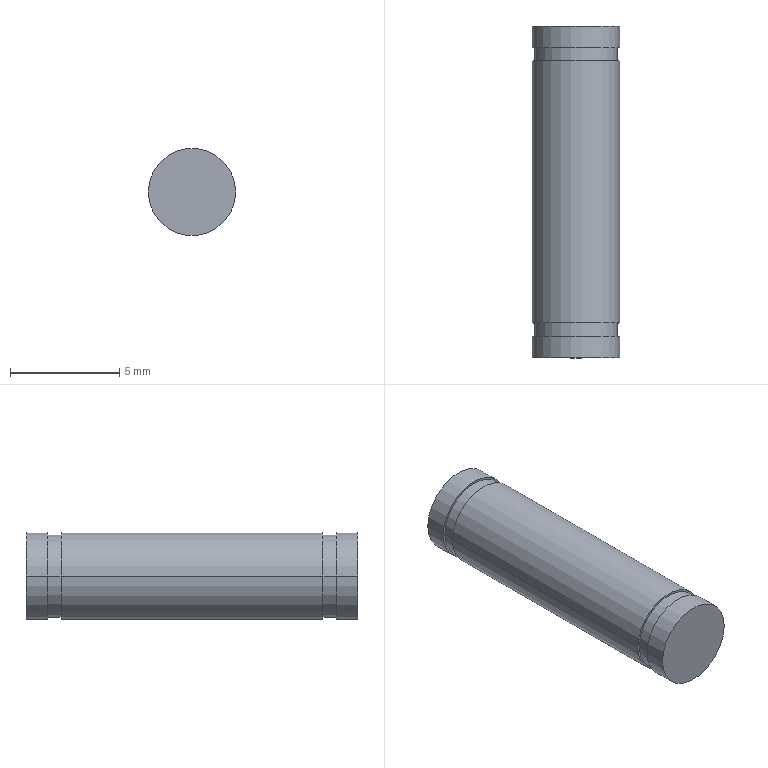Part | SolidWorks | features Revolution 1 | 1 solid | 16 faces | box 4 x 15.2 x 4 mm | volume 189.539 mm3 | cylinder 10 | plane 6 | commonest cylinder face diameters 4 x6 3.8 x4
STEP:
#1=CARTESIAN_POINT('',(-0.002,-0.01255,0.));
#2=VERTEX_POINT('',#1);
#3=CARTESIAN_POINT('',(0.002,-0.01255,0.));
#4=VERTEX_POINT('',#3);
#5=CARTESIAN_POINT('',(0.,-0.01255,0.));
#6=DIRECTION('',(0.,1.,0.));
#7=DIRECTION('',(-1.,0.,0.));
#8=AXIS2_PLACEMENT_3D('',#5,#6,#7);
#9=CIRCLE('',#8,0.002);
#10=EDGE_CURVE('',#2,#4,#9,.T.);
#11=ORIENTED_EDGE('',*,*,#10,.T.);
#12=CARTESIAN_POINT('',(0.002,-0.01155,0.));
#13=VERTEX_POINT('',#12);
#14=CARTESIAN_POINT('',(0.002,0.002647,0.));
#15=DIRECTION('',(0.,1.,0.));
#16=VECTOR('',#15,1.);
#17=LINE('',#14,#16);
#18=EDGE_CURVE('',#4,#13,#17,.T.);
#19=ORIENTED_EDGE('',*,*,#18,.T.);
#20=CARTESIAN_POINT('',(-0.002,-0.01155,0.));
#21=VERTEX_POINT('',#20);
#22=CARTESIAN_POINT('',(0.,-0.01155,0.));
#23=DIRECTION('',(0.,1.,0.));
#24=DIRECTION('',(-1.,0.,0.));
#25=AXIS2_PLACEMENT_3D('',#22,#23,#24);
#26=CIRCLE('',#25,0.002);
#27=EDGE_CURVE('',#21,#13,#26,.T.);
#28=ORIENTED_EDGE('',*,*,#27,.F.);
#29=CARTESIAN_POINT('',(-0.002,0.002647,0.));
#30=DIRECTION('',(0.,1.,0.));
#31=VECTOR('',#30,1.);
#32=LINE('',#29,#31);
#33=EDGE_CURVE('',#2,#21,#32,.T.);
#34=ORIENTED_EDGE('',*,*,#33,.F.);
#35=EDGE_LOOP('',(#11,#19,#28,#34));
#36=FACE_OUTER_BOUND('',#35,.T.);
#37=CARTESIAN_POINT('',(0.,0.002647,0.));
#38=DIRECTION('',(0.,1.,0.));
#39=DIRECTION('',(-1.,0.,0.));
#40=AXIS2_PLACEMENT_3D('',#37,#38,#39);
#41=CYLINDRICAL_SURFACE('',#40,0.002);
#42=ADVANCED_FACE('',(#36),#41,.T.);
#43=CARTESIAN_POINT('',(-0.0019,-0.01155,0.));
#44=VERTEX_POINT('',#43);
#45=CARTESIAN_POINT('',(0.0019,-0.01155,0.));
#46=VERTEX_POINT('',#45);
#47=CARTESIAN_POINT('',(0.,-0.01155,0.));
#48=DIRECTION('',(0.,1.,0.));
#49=DIRECTION('',(-1.,0.,0.));
#50=AXIS2_PLACEMENT_3D('',#47,#48,#49);
#51=CIRCLE('',#50,0.0019);
#52=EDGE_CURVE('',#44,#46,#51,.T.);
#53=ORIENTED_EDGE('',*,*,#52,.T.);
#54=CARTESIAN_POINT('',(0.0019,-0.01095,0.));
#55=VERTEX_POINT('',#54);
#56=CARTESIAN_POINT('',(0.0019,0.002647,0.));
#57=DIRECTION('',(0.,1.,0.));
#58=VECTOR('',#57,1.);
#59=LINE('',#56,#58);
#60=EDGE_CURVE('',#46,#55,#59,.T.);
#61=ORIENTED_EDGE('',*,*,#60,.T.);
#62=CARTESIAN_POINT('',(-0.0019,-0.01095,0.));
#63=VERTEX_POINT('',#62);
#64=CARTESIAN_POINT('',(0.,-0.01095,0.));
#65=DIRECTION('',(0.,1.,0.));
#66=DIRECTION('',(-1.,0.,0.));
#67=AXIS2_PLACEMENT_3D('',#64,#65,#66);
#68=CIRCLE('',#67,0.0019);
#69=EDGE_CURVE('',#63,#55,#68,.T.);
#70=ORIENTED_EDGE('',*,*,#69,.F.);
#71=CARTESIAN_POINT('',(-0.0019,0.002647,0.));
#72=DIRECTION('',(0.,1.,0.));
#73=VECTOR('',#72,1.);
#74=LINE('',#71,#73);
#75=EDGE_CURVE('',#44,#63,#74,.T.);
#76=ORIENTED_EDGE('',*,*,#75,.F.);
#77=EDGE_LOOP('',(#53,#61,#70,#76));
#78=FACE_OUTER_BOUND('',#77,.T.);
#79=CARTESIAN_POINT('',(0.,0.002647,0.));
#80=DIRECTION('',(0.,1.,0.));
#81=DIRECTION('',(-1.,0.,0.));
#82=AXIS2_PLACEMENT_3D('',#79,#80,#81);
#83=CYLINDRICAL_SURFACE('',#82,0.0019);
#84=ADVANCED_FACE('',(#78),#83,.T.);
#85=CARTESIAN_POINT('',(-0.002,-0.01095,0.));
#86=VERTEX_POINT('',#85);
#87=CARTESIAN_POINT('',(0.002,-0.01095,0.));
#88=VERTEX_POINT('',#87);
#89=CARTESIAN_POINT('',(0.,-0.01095,0.));
#90=DIRECTION('',(0.,1.,0.));
#91=DIRECTION('',(-1.,0.,0.));
#92=AXIS2_PLACEMENT_3D('',#89,#90,#91);
#93=CIRCLE('',#92,0.002);
#94=EDGE_CURVE('',#86,#88,#93,.T.);
#95=ORIENTED_EDGE('',*,*,#94,.T.);
#96=CARTESIAN_POINT('',(0.002,0.001047,0.));
#97=VERTEX_POINT('',#96);
#98=CARTESIAN_POINT('',(0.002,0.002647,0.));
#99=DIRECTION('',(0.,1.,0.));
#100=VECTOR('',#99,1.);
#101=LINE('',#98,#100);
#102=EDGE_CURVE('',#88,#97,#101,.T.);
#103=ORIENTED_EDGE('',*,*,#102,.T.);
#104=CARTESIAN_POINT('',(-0.002,0.001047,0.));
#105=VERTEX_POINT('',#104);
#106=CARTESIAN_POINT('',(0.,0.001047,0.));
#107=DIRECTION('',(0.,1.,0.));
#108=DIRECTION('',(-1.,0.,0.));
#109=AXIS2_PLACEMENT_3D('',#106,#107,#108);
#110=CIRCLE('',#109,0.002);
#111=EDGE_CURVE('',#105,#97,#110,.T.);
#112=ORIENTED_EDGE('',*,*,#111,.F.);
#113=CARTESIAN_POINT('',(-0.002,0.002647,0.));
#114=DIRECTION('',(0.,1.,0.));
#115=VECTOR('',#114,1.);
#116=LINE('',#113,#115);
#117=EDGE_CURVE('',#86,#105,#116,.T.);
#118=ORIENTED_EDGE('',*,*,#117,.F.);
#119=EDGE_LOOP('',(#95,#103,#112,#118));
#120=FACE_OUTER_BOUND('',#119,.T.);
#121=CARTESIAN_POINT('',(0.,0.002647,0.));
#122=DIRECTION('',(0.,1.,0.));
#123=DIRECTION('',(-1.,0.,0.));
#124=AXIS2_PLACEMENT_3D('',#121,#122,#123);
#125=CYLINDRICAL_SURFACE('',#124,0.002);
#126=ADVANCED_FACE('',(#120),#125,.T.);
#127=CARTESIAN_POINT('',(-0.0019,0.001047,0.));
#128=VERTEX_POINT('',#127);
#129=CARTESIAN_POINT('',(0.0019,0.001047,0.));
#130=VERTEX_POINT('',#129);
#131=CARTESIAN_POINT('',(0.,0.001047,0.));
#132=DIRECTION('',(0.,1.,0.));
#133=DIRECTION('',(-1.,0.,0.));
#134=AXIS2_PLACEMENT_3D('',#131,#132,#133);
#135=CIRCLE('',#134,0.0019);
#136=EDGE_CURVE('',#128,#130,#135,.T.);
#137=ORIENTED_EDGE('',*,*,#136,.T.);
#138=CARTESIAN_POINT('',(0.0019,0.001647,0.));
#139=VERTEX_POINT('',#138);
#140=CARTESIAN_POINT('',(0.0019,0.002647,0.));
#141=DIRECTION('',(0.,1.,0.));
#142=VECTOR('',#141,1.);
#143=LINE('',#140,#142);
#144=EDGE_CURVE('',#130,#139,#143,.T.);
#145=ORIENTED_EDGE('',*,*,#144,.T.);
#146=CARTESIAN_POINT('',(-0.0019,0.001647,0.));
#147=VERTEX_POINT('',#146);
#148=CARTESIAN_POINT('',(0.,0.001647,0.));
#149=DIRECTION('',(0.,1.,0.));
#150=DIRECTION('',(-1.,0.,0.));
#151=AXIS2_PLACEMENT_3D('',#148,#149,#150);
#152=CIRCLE('',#151,0.0019);
#153=EDGE_CURVE('',#147,#139,#152,.T.);
#154=ORIENTED_EDGE('',*,*,#153,.F.);
#155=CARTESIAN_POINT('',(-0.0019,0.002647,0.));
#156=DIRECTION('',(0.,1.,0.));
#157=VECTOR('',#156,1.);
#158=LINE('',#155,#157);
#159=EDGE_CURVE('',#128,#147,#158,.T.);
#160=ORIENTED_EDGE('',*,*,#159,.F.);
#161=EDGE_LOOP('',(#137,#145,#154,#160));
#162=FACE_OUTER_BOUND('',#161,.T.);
#163=CARTESIAN_POINT('',(0.,0.002647,0.));
#164=DIRECTION('',(0.,1.,0.));
#165=DIRECTION('',(-1.,0.,0.));
#166=AXIS2_PLACEMENT_3D('',#163,#164,#165);
#167=CYLINDRICAL_SURFACE('',#166,0.0019);
#168=ADVANCED_FACE('',(#162),#167,.T.);
#169=CARTESIAN_POINT('',(-0.002,0.001647,0.));
#170=VERTEX_POINT('',#169);
#171=CARTESIAN_POINT('',(0.002,0.001647,0.));
#172=VERTEX_POINT('',#171);
#173=CARTESIAN_POINT('',(0.,0.001647,0.));
#174=DIRECTION('',(0.,1.,0.));
#175=DIRECTION('',(-1.,0.,0.));
#176=AXIS2_PLACEMENT_3D('',#173,#174,#175);
#177=CIRCLE('',#176,0.002);
#178=EDGE_CURVE('',#170,#172,#177,.T.);
#179=ORIENTED_EDGE('',*,*,#178,.T.);
#180=CARTESIAN_POINT('',(0.002,0.002647,0.));
#181=VERTEX_POINT('',#180);
#182=CARTESIAN_POINT('',(0.002,0.002647,0.));
#183=DIRECTION('',(0.,1.,0.));
#184=VECTOR('',#183,1.);
#185=LINE('',#182,#184);
#186=EDGE_CURVE('',#172,#181,#185,.T.);
#187=ORIENTED_EDGE('',*,*,#186,.T.);
#188=CARTESIAN_POINT('',(-0.002,0.002647,0.));
#189=VERTEX_POINT('',#188);
#190=CARTESIAN_POINT('',(0.,0.002647,0.));
#191=DIRECTION('',(0.,1.,0.));
#192=DIRECTION('',(-1.,0.,0.));
#193=AXIS2_PLACEMENT_3D('',#190,#191,#192);
#194=CIRCLE('',#193,0.002);
#195=EDGE_CURVE('',#189,#181,#194,.T.);
#196=ORIENTED_EDGE('',*,*,#195,.F.);
#197=CARTESIAN_POINT('',(-0.002,0.002647,0.));
#198=DIRECTION('',(0.,1.,0.));
#199=VECTOR('',#198,1.);
#200=LINE('',#197,#199);
#201=EDGE_CURVE('',#170,#189,#200,.T.);
#202=ORIENTED_EDGE('',*,*,#201,.F.);
#203=EDGE_LOOP('',(#179,#187,#196,#202));
#204=FACE_OUTER_BOUND('',#203,.T.);
#205=CARTESIAN_POINT('',(0.,0.002647,0.));
#206=DIRECTION('',(0.,1.,0.));
#207=DIRECTION('',(-1.,0.,0.));
#208=AXIS2_PLACEMENT_3D('',#205,#206,#207);
#209=CYLINDRICAL_SURFACE('',#208,0.002);
#210=ADVANCED_FACE('',(#204),#209,.T.);
#211=ORIENTED_EDGE('',*,*,#195,.T.);
#212=CARTESIAN_POINT('',(0.,0.002647,0.));
#213=DIRECTION('',(0.,1.,0.));
#214=DIRECTION('',(-1.,0.,0.));
#215=AXIS2_PLACEMENT_3D('',#212,#213,#214);
#216=CIRCLE('',#215,0.002);
#217=EDGE_CURVE('',#181,#189,#216,.T.);
#218=ORIENTED_EDGE('',*,*,#217,.T.);
#219=EDGE_LOOP('',(#211,#218));
#220=FACE_OUTER_BOUND('',#219,.T.);
#221=CARTESIAN_POINT('',(0.,0.002647,0.));
#222=DIRECTION('',(0.,-1.,0.));
#223=DIRECTION('',(1.,0.,0.));
#224=AXIS2_PLACEMENT_3D('',#221,#222,#223);
#225=PLANE('',#224);
#226=ADVANCED_FACE('',(#220),#225,.F.);
#227=ORIENTED_EDGE('',*,*,#186,.F.);
#228=CARTESIAN_POINT('',(0.,0.001647,0.));
#229=DIRECTION('',(0.,1.,0.));
#230=DIRECTION('',(-1.,0.,0.));
#231=AXIS2_PLACEMENT_3D('',#228,#229,#230);
#232=CIRCLE('',#231,0.002);
#233=EDGE_CURVE('',#172,#170,#232,.T.);
#234=ORIENTED_EDGE('',*,*,#233,.T.);
#235=ORIENTED_EDGE('',*,*,#201,.T.);
#236=ORIENTED_EDGE('',*,*,#217,.F.);
#237=EDGE_LOOP('',(#227,#234,#235,#236));
#238=FACE_OUTER_BOUND('',#237,.T.);
#239=CARTESIAN_POINT('',(0.,0.002647,0.));
#240=DIRECTION('',(0.,1.,0.));
#241=DIRECTION('',(-1.,0.,0.));
#242=AXIS2_PLACEMENT_3D('',#239,#240,#241);
#243=CYLINDRICAL_SURFACE('',#242,0.002);
#244=ADVANCED_FACE('',(#238),#243,.T.);
#245=ORIENTED_EDGE('',*,*,#178,.F.);
#246=ORIENTED_EDGE('',*,*,#233,.F.);
#247=EDGE_LOOP('',(#245,#246));
#248=FACE_OUTER_BOUND('',#247,.T.);
#249=ORIENTED_EDGE('',*,*,#153,.T.);
#250=CARTESIAN_POINT('',(0.,0.001647,0.));
#251=DIRECTION('',(0.,1.,0.));
#252=DIRECTION('',(-1.,0.,0.));
#253=AXIS2_PLACEMENT_3D('',#250,#251,#252);
#254=CIRCLE('',#253,0.0019);
#255=EDGE_CURVE('',#139,#147,#254,.T.);
#256=ORIENTED_EDGE('',*,*,#255,.T.);
#257=EDGE_LOOP('',(#249,#256));
#258=FACE_BOUND('',#257,.T.);
#259=CARTESIAN_POINT('',(0.002,0.001647,0.));
#260=DIRECTION('',(0.,1.,0.));
#261=DIRECTION('',(-1.,0.,0.));
#262=AXIS2_PLACEMENT_3D('',#259,#260,#261);
#263=PLANE('',#262);
#264=ADVANCED_FACE('',(#248,#258),#263,.F.);
#265=ORIENTED_EDGE('',*,*,#144,.F.);
#266=CARTESIAN_POINT('',(0.,0.001047,0.));
#267=DIRECTION('',(0.,1.,0.));
#268=DIRECTION('',(-1.,0.,0.));
#269=AXIS2_PLACEMENT_3D('',#266,#267,#268);
#270=CIRCLE('',#269,0.0019);
#271=EDGE_CURVE('',#130,#128,#270,.T.);
#272=ORIENTED_EDGE('',*,*,#271,.T.);
#273=ORIENTED_EDGE('',*,*,#159,.T.);
#274=ORIENTED_EDGE('',*,*,#255,.F.);
#275=EDGE_LOOP('',(#265,#272,#273,#274));
#276=FACE_OUTER_BOUND('',#275,.T.);
#277=CARTESIAN_POINT('',(0.,0.002647,0.));
#278=DIRECTION('',(0.,1.,0.));
#279=DIRECTION('',(-1.,0.,0.));
#280=AXIS2_PLACEMENT_3D('',#277,#278,#279);
#281=CYLINDRICAL_SURFACE('',#280,0.0019);
#282=ADVANCED_FACE('',(#276),#281,.T.);
#283=ORIENTED_EDGE('',*,*,#136,.F.);
#284=ORIENTED_EDGE('',*,*,#271,.F.);
#285=EDGE_LOOP('',(#283,#284));
#286=FACE_BOUND('',#285,.T.);
#287=ORIENTED_EDGE('',*,*,#111,.T.);
#288=CARTESIAN_POINT('',(0.,0.001047,0.));
#289=DIRECTION('',(0.,1.,0.));
#290=DIRECTION('',(-1.,0.,0.));
#291=AXIS2_PLACEMENT_3D('',#288,#289,#290);
#292=CIRCLE('',#291,0.002);
#293=EDGE_CURVE('',#97,#105,#292,.T.);
#294=ORIENTED_EDGE('',*,*,#293,.T.);
#295=EDGE_LOOP('',(#287,#294));
#296=FACE_OUTER_BOUND('',#295,.T.);
#297=CARTESIAN_POINT('',(0.0019,0.001047,0.));
#298=DIRECTION('',(0.,-1.,0.));
#299=DIRECTION('',(1.,0.,0.));
#300=AXIS2_PLACEMENT_3D('',#297,#298,#299);
#301=PLANE('',#300);
#302=ADVANCED_FACE('',(#286,#296),#301,.F.);
#303=ORIENTED_EDGE('',*,*,#102,.F.);
#304=CARTESIAN_POINT('',(0.,-0.01095,0.));
#305=DIRECTION('',(0.,1.,0.));
#306=DIRECTION('',(-1.,0.,0.));
#307=AXIS2_PLACEMENT_3D('',#304,#305,#306);
#308=CIRCLE('',#307,0.002);
#309=EDGE_CURVE('',#88,#86,#308,.T.);
#310=ORIENTED_EDGE('',*,*,#309,.T.);
#311=ORIENTED_EDGE('',*,*,#117,.T.);
#312=ORIENTED_EDGE('',*,*,#293,.F.);
#313=EDGE_LOOP('',(#303,#310,#311,#312));
#314=FACE_OUTER_BOUND('',#313,.T.);
#315=CARTESIAN_POINT('',(0.,0.002647,0.));
#316=DIRECTION('',(0.,1.,0.));
#317=DIRECTION('',(-1.,0.,0.));
#318=AXIS2_PLACEMENT_3D('',#315,#316,#317);
#319=CYLINDRICAL_SURFACE('',#318,0.002);
#320=ADVANCED_FACE('',(#314),#319,.T.);
#321=ORIENTED_EDGE('',*,*,#94,.F.);
#322=ORIENTED_EDGE('',*,*,#309,.F.);
#323=EDGE_LOOP('',(#321,#322));
#324=FACE_OUTER_BOUND('',#323,.T.);
#325=ORIENTED_EDGE('',*,*,#69,.T.);
#326=CARTESIAN_POINT('',(0.,-0.01095,0.));
#327=DIRECTION('',(0.,1.,0.));
#328=DIRECTION('',(-1.,0.,0.));
#329=AXIS2_PLACEMENT_3D('',#326,#327,#328);
#330=CIRCLE('',#329,0.0019);
#331=EDGE_CURVE('',#55,#63,#330,.T.);
#332=ORIENTED_EDGE('',*,*,#331,.T.);
#333=EDGE_LOOP('',(#325,#332));
#334=FACE_BOUND('',#333,.T.);
#335=CARTESIAN_POINT('',(0.002,-0.01095,0.));
#336=DIRECTION('',(0.,1.,0.));
#337=DIRECTION('',(-1.,0.,0.));
#338=AXIS2_PLACEMENT_3D('',#335,#336,#337);
#339=PLANE('',#338);
#340=ADVANCED_FACE('',(#324,#334),#339,.F.);
#341=ORIENTED_EDGE('',*,*,#60,.F.);
#342=CARTESIAN_POINT('',(0.,-0.01155,0.));
#343=DIRECTION('',(0.,1.,0.));
#344=DIRECTION('',(-1.,0.,0.));
#345=AXIS2_PLACEMENT_3D('',#342,#343,#344);
#346=CIRCLE('',#345,0.0019);
#347=EDGE_CURVE('',#46,#44,#346,.T.);
#348=ORIENTED_EDGE('',*,*,#347,.T.);
#349=ORIENTED_EDGE('',*,*,#75,.T.);
#350=ORIENTED_EDGE('',*,*,#331,.F.);
#351=EDGE_LOOP('',(#341,#348,#349,#350));
#352=FACE_OUTER_BOUND('',#351,.T.);
#353=CARTESIAN_POINT('',(0.,0.002647,0.));
#354=DIRECTION('',(0.,1.,0.));
#355=DIRECTION('',(-1.,0.,0.));
#356=AXIS2_PLACEMENT_3D('',#353,#354,#355);
#357=CYLINDRICAL_SURFACE('',#356,0.0019);
#358=ADVANCED_FACE('',(#352),#357,.T.);
#359=ORIENTED_EDGE('',*,*,#52,.F.);
#360=ORIENTED_EDGE('',*,*,#347,.F.);
#361=EDGE_LOOP('',(#359,#360));
#362=FACE_BOUND('',#361,.T.);
#363=ORIENTED_EDGE('',*,*,#27,.T.);
#364=CARTESIAN_POINT('',(0.,-0.01155,0.));
#365=DIRECTION('',(0.,1.,0.));
#366=DIRECTION('',(-1.,0.,0.));
#367=AXIS2_PLACEMENT_3D('',#364,#365,#366);
#368=CIRCLE('',#367,0.002);
#369=EDGE_CURVE('',#13,#21,#368,.T.);
#370=ORIENTED_EDGE('',*,*,#369,.T.);
#371=EDGE_LOOP('',(#363,#370));
#372=FACE_OUTER_BOUND('',#371,.T.);
#373=CARTESIAN_POINT('',(0.0019,-0.01155,0.));
#374=DIRECTION('',(0.,-1.,0.));
#375=DIRECTION('',(1.,0.,0.));
#376=AXIS2_PLACEMENT_3D('',#373,#374,#375);
#377=PLANE('',#376);
#378=ADVANCED_FACE('',(#362,#372),#377,.F.);
#379=ORIENTED_EDGE('',*,*,#18,.F.);
#380=CARTESIAN_POINT('',(0.,-0.01255,0.));
#381=DIRECTION('',(0.,1.,0.));
#382=DIRECTION('',(-1.,0.,0.));
#383=AXIS2_PLACEMENT_3D('',#380,#381,#382);
#384=CIRCLE('',#383,0.002);
#385=EDGE_CURVE('',#4,#2,#384,.T.);
#386=ORIENTED_EDGE('',*,*,#385,.T.);
#387=ORIENTED_EDGE('',*,*,#33,.T.);
#388=ORIENTED_EDGE('',*,*,#369,.F.);
#389=EDGE_LOOP('',(#379,#386,#387,#388));
#390=FACE_OUTER_BOUND('',#389,.T.);
#391=CARTESIAN_POINT('',(0.,0.002647,0.));
#392=DIRECTION('',(0.,1.,0.));
#393=DIRECTION('',(-1.,0.,0.));
#394=AXIS2_PLACEMENT_3D('',#391,#392,#393);
#395=CYLINDRICAL_SURFACE('',#394,0.002);
#396=ADVANCED_FACE('',(#390),#395,.T.);
#397=ORIENTED_EDGE('',*,*,#10,.F.);
#398=ORIENTED_EDGE('',*,*,#385,.F.);
#399=EDGE_LOOP('',(#397,#398));
#400=FACE_OUTER_BOUND('',#399,.T.);
#401=CARTESIAN_POINT('',(0.002,-0.01255,0.));
#402=DIRECTION('',(0.,1.,0.));
#403=DIRECTION('',(-1.,0.,0.));
#404=AXIS2_PLACEMENT_3D('',#401,#402,#403);
#405=PLANE('',#404);
#406=ADVANCED_FACE('',(#400),#405,.F.);
#407=CLOSED_SHELL('',(#42,#84,#126,#168,#210,#226,#244,#264,#282,#302,#320,#340,#358,#378,#396,#406));
#408=MANIFOLD_SOLID_BREP('',#407);
#409=CARTESIAN_POINT('',(0.,0.,0.));
#410=DIRECTION('',(0.,0.,1.));
#411=DIRECTION('',(1.,0.,0.));
#412=AXIS2_PLACEMENT_3D('',#409,#410,#411);
#413=(LENGTH_UNIT()NAMED_UNIT(*)SI_UNIT($,.METRE.));
#414=UNCERTAINTY_MEASURE_WITH_UNIT(LENGTH_MEASURE(0.00001),#413,'','');
#415=(NAMED_UNIT(*)PLANE_ANGLE_UNIT()SI_UNIT($,.RADIAN.));
#416=(NAMED_UNIT(*)SI_UNIT($,.STERADIAN.)SOLID_ANGLE_UNIT());
#417=(GEOMETRIC_REPRESENTATION_CONTEXT(3)GLOBAL_UNCERTAINTY_ASSIGNED_CONTEXT((#414))GLOBAL_UNIT_ASSIGNED_CONTEXT((#413,#415,#416))REPRESENTATION_CONTEXT('',''));
#418=ADVANCED_BREP_SHAPE_REPRESENTATION('',(#408,#412),#417);